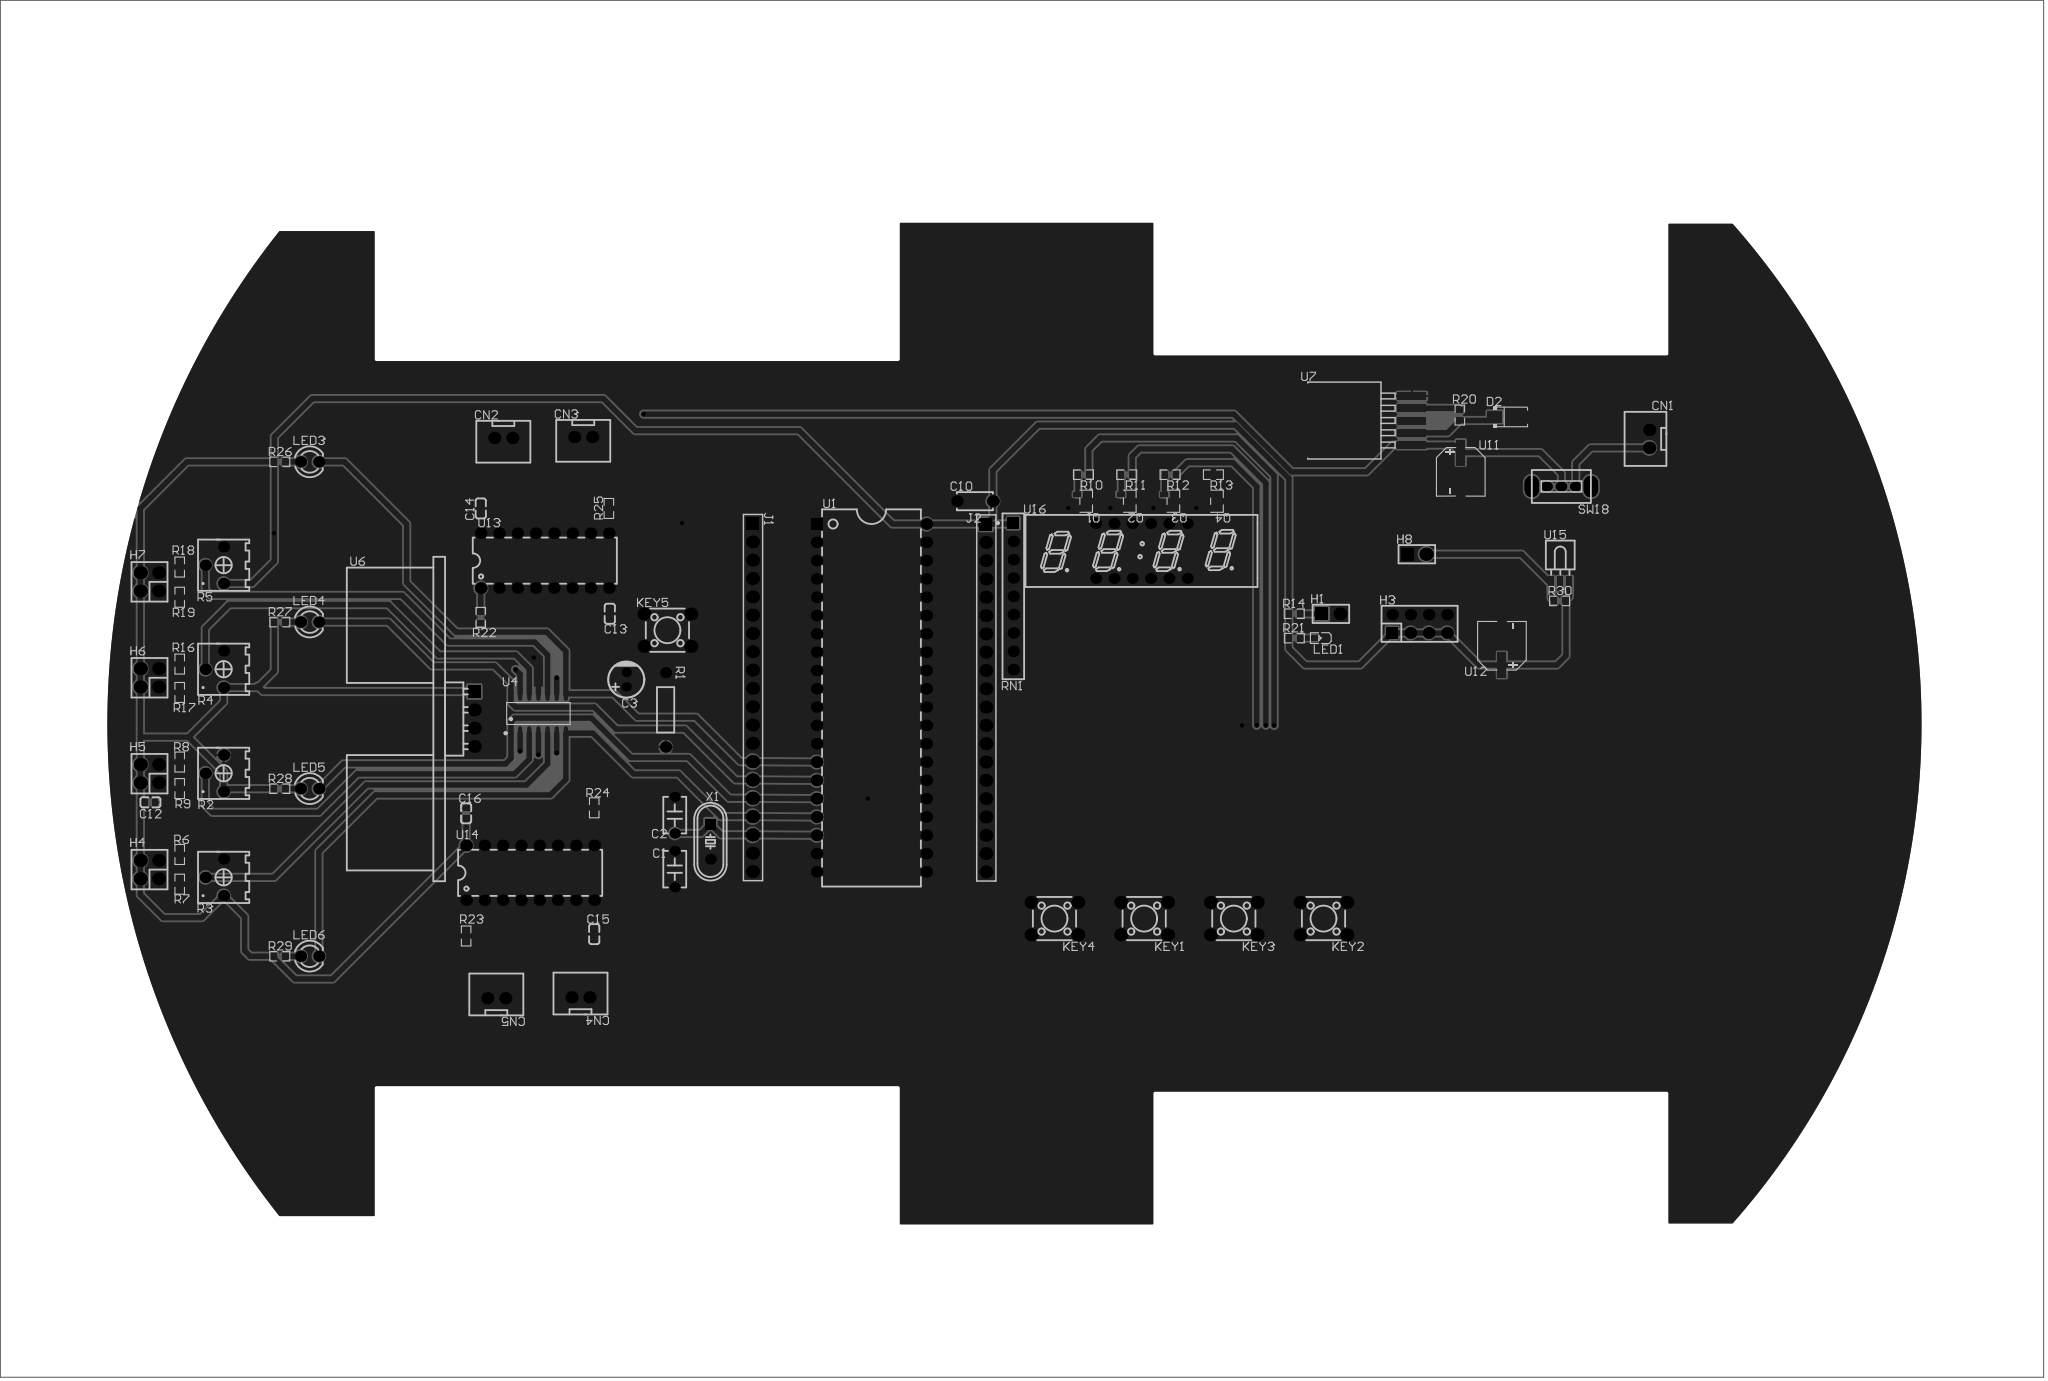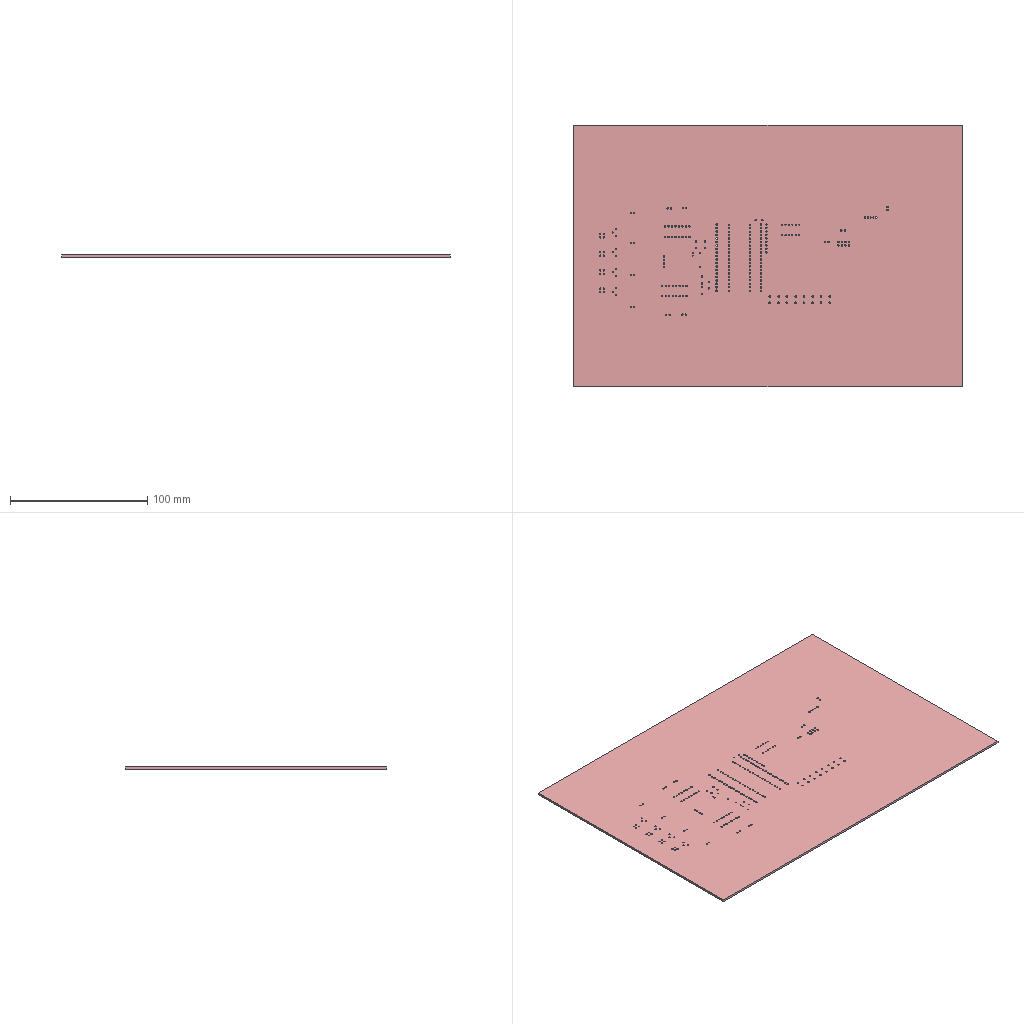Circuit board layout | Altium Designer | box 283.6 x 191 x 1.6 mm
Layer stack:
# Altium Designer layer stack of  (unit mm; dielectric type: 0 none, 1 core, 2 prepreg, 3 surface material)
index,name,kind,layer,copper_thickness_mm,dielectric_type,dielectric_thickness_mm,dielectric_material,dielectric_constant
0,Top Paste Mask Layer,other,,,,,,
1,Top Silkscreen Layer,other,,,,,,
2,Top Solder Mask Layer,dielectric,,,3,0.01,,3.3
3,Top Layer,copper,Top Layer,0.035,,,,
4,Dielectric1,dielectric,,,3,1.51,FR4,4.5
5,Bottom Layer,copper,Bottom Layer,0.035,,,,
6,Bottom Solder Mask Layer,dielectric,,,3,0.01,,3.3
7,Bottom Silkscreen Layer,other,,,,,,
8,Bottom Paste Mask Layer,other,,,,,,
# drill layer pairs: low layer,high layer
drill_pair,Top Layer,Bottom Layer
Part placement:
Designator,Comment,Layer,Footprint,Center-X(mm),Center-Y(mm),Rotation
C1,,TopLayer,CAP-TH_L5.0-W2.5-P5.08-D0.7,163.449,140.335,270
C2,,TopLayer,CAP-TH_L5.0-W2.5-P5.08-D0.7,163.449,147.828,90
C3,,TopLayer,CAP-TH_BD5.0-P2.00-D0.8-FD,156.718,166.624,90
C10,,TopLayer,CAP-TH_L5.0-W2.5-P5.00-D1.0,205.105,191.389,0
C12,104,TopLayer,C0603,90.678,149.606,0
C13,100nF,TopLayer,C0603,154.432,175.768,270
C14,100nF,TopLayer,C0603,136.525,190.373,90
C15,100nF,TopLayer,C0603,152.273,131.318,270
C16,100nF,TopLayer,C0603,134.493,148.082,90
CN1,XH2.54*2P_through-hole,TopLayer,CONN-TH_2P-P2.50-XH2.54-2P,298.704,200.025,270
CN2,XH2.54*2P_through-hole,TopLayer,CONN-TH_2P-P2.50-XH2.54-2P,139.658,200.155,0
CN3,XH2.54*2P_through-hole,TopLayer,CONN-TH_2P-P2.50-XH2.54-2P,150.749,200.279,0
CN4,XH2.54*2P_through-hole,TopLayer,CONN-TH_2P-P2.50-XH2.54-2P,150.368,122.555,180
CN5,XH2.54*2P_through-hole,TopLayer,CONN-TH_2P-P2.50-XH2.54-2P,138.684,122.428,180
D2,SS34,TopLayer,SMA_L4.3-W2.6-LS5.0-RD,279.654,203.073,0
H1,,TopLayer,HDR-TH_2P-P2.54-V-M-1,254.519,175.748,0
H3,,TopLayer,HDR-TH_8P-P2.54-V-F-R2-C4-S2.54-1,266.827,174.371,0
H4,,TopLayer,HDR-TH_4P-P2.54-V-F-R2-C2-S2.54,90.548,140.271,90
H5,,TopLayer,HDR-TH_4P-P2.54-V-F-R2-C2-S2.54,90.548,153.577,90
H6,,TopLayer,HDR-TH_4P-P2.54-V-F-R2-C2-S2.54,90.548,166.884,90
H7,,TopLayer,HDR-TH_4P-P2.54-V-F-R2-C2-S2.54,90.548,180.19,90
H8,,TopLayer,HDR-TH_2P-P2.54-V-M-1,266.446,184.023,0
J1,,TopLayer,HDR-TH_20P-P2.54-V-M-1,174.248,164.14,270
J2,,TopLayer,HDR-TH_20P-P2.54-V-M-1,206.629,164.084,270
KEY1,UK-B0202-G5-160,TopLayer,SW-TH_4P-L6.0-W6.0-P4.50-LS6.5,228.6,133.477,180
KEY2,UK-B0202-G5-160,TopLayer,SW-TH_4P-L6.0-W6.0-P4.50-LS6.5,253.492,133.477,180
KEY3,UK-B0202-G5-160,TopLayer,SW-TH_4P-L6.0-W6.0-P4.50-LS6.5,241.046,133.477,180
KEY4,UK-B0202-G5-160,TopLayer,SW-TH_4P-L6.0-W6.0-P4.50-LS6.5,216.154,133.477,180
KEY5,UK-B0202-G5-160,TopLayer,SW-TH_4P-L6.0-W6.0-P4.50-LS6.5,162.433,173.482,0
LED1,,TopLayer,LED_0603,253.066,172.39,180
LED3,,TopLayer,LED-TH_BD3.0-P2.54-FD,112.789,196.835,0
LED4,,TopLayer,LED-TH_BD3.0-P2.54-FD,112.789,174.61,0
LED5,,TopLayer,LED-TH_BD3.0-P2.54-FD,112.789,151.496,0
LED6,,TopLayer,LED-TH_BD3.0-P2.54-FD,112.789,128.255,0
Q1,S8550,TopLayer,SOT-23-3_L2.9-W1.6-P1.90-LS2.8-BR,220.553,191.376,180
Q2,S8550,TopLayer,SOT-23-3_L2.9-W1.6-P1.90-LS2.8-BR,226.604,191.376,180
Q3,S8550,TopLayer,SOT-23-3_L2.9-W1.6-P1.90-LS2.8-BR,232.655,191.376,180
Q4,S8550,TopLayer,SOT-23-3_L2.9-W1.6-P1.90-LS2.8-BR,238.705,191.376,180
R1,,TopLayer,RES-TH_BD2.4-L6.3-P10.30-D0.6,162.179,162.433,270
R2,-,TopLayer,RES-ADJ-TH_3362P,99.568,153.628,90
R3,-,TopLayer,RES-ADJ-TH_3362P,99.568,139.192,90
R4,-,TopLayer,RES-ADJ-TH_3362P,99.568,168.063,90
R5,-,TopLayer,RES-ADJ-TH_3362P,99.568,182.499,90
R6,10K,TopLayer,R0603,94.742,142.367,90
R7,100,TopLayer,R0603,94.742,138.25,270
R8,10K,TopLayer,R0603,94.742,155.194,90
R9,100,TopLayer,R0603,94.742,151.511,270
R10,1K,TopLayer,R0603,220.172,195.059,180
R11,1K,TopLayer,R0603,226.184,195.059,180
R12,1K,TopLayer,R0603,232.196,195.059,180
R13,1K,TopLayer,R0603,238.208,195.059,180
R14,33,TopLayer,R0603,249.428,175.768,0
R16,10K,TopLayer,R0603,94.742,168.783,90
R17,100,TopLayer,R0603,94.742,164.846,270
R18,10K,TopLayer,R0603,94.742,182.245,90
R19,100,TopLayer,R0603,94.742,178.054,270
R20,33U,TopLayer,R0603,272.415,203.327,270
R21,2K,TopLayer,R0603,249.44,172.383,0
R22,1K,TopLayer,R0603,136.525,175.26,90
R23,1K,TopLayer,R0603,134.493,131.064,90
R24,1K,TopLayer,R0603,152.273,148.844,90
R25,1K,TopLayer,R0603,154.305,190.373,90
R26,1K,TopLayer,R0603,108.636,196.835,0
R27,1K,TopLayer,R0603,108.636,174.61,0
R28,1K,TopLayer,R0603,108.636,151.496,0
R29,1K,TopLayer,R0603,108.636,128.255,0
R30,10K,TopLayer,R0603,286.258,177.546,0
RN1,,TopLayer,RES-ARRAY-TH_9P-P2.54-D1.0,210.439,178.181,270
SW18,,TopLayer,拨动开关,286.504,193.421,180
U1,,TopLayer,DIP-40_L52.0-W13.7-P2.54-LS15.2-BL,190.754,164.084,270
U4,LM324NLM324,TopLayer,SOP-14_L8.6-W3.9-P1.27-LS6.0-BL,144.526,161.925,0
U6,HC-SR04,TopLayer,TH_HC-SR04V,135.636,161.163,270
U7,LM2596SX-5.0/NOPB-YJLTY,TopLayer,TO-263-5_L10.0-W8.4-P1.70-LS15.3-BR,260.223,202.565,0
U11,220uF,TopLayer,CAP-SMD_BD6.3-L6.6-W6.6-LS7.2-FD,272.542,195.453,270
U12,220uF,TopLayer,CAP-SMD_BD6.3-L6.6-W6.6-LS7.2-FD,278.258,171.323,90
U13,L293D,TopLayer,DIP-16_L20.0-W6.4-P2.54-LS7.6-BL,145.415,183.134,0
U14,L293D,TopLayer,DIP-16_L20.0-W6.4-P2.54-LS7.6-BL,143.383,139.827,0
U15,CH0038A_38B/5*5mm/infrared receiver,TopLayer,OPTO-SMD_CH0038A_38B,286.35,179.917,0
U16,0.28 4-digit display,TopLayer,LED-SEG-TH_12P-L32.1-W10.0-P12.7-S7.62-BL,228.23,184.478,0
X1,,TopLayer,HC-49US_L11.5-W4.5-P4.88,168.402,144.145,270
Pad and via stacks:
# Altium Designer via and pad stacks of  (unit mm). Each distinct definition once, with the count of objects using it.
# via: kind,start_layer,end_layer,hole_mm,diameter_mm,mode(0 simple;1 top-mid-bottom;2 full stack),diameter_per_layer,count,example_net
# pad: kind,layer,hole_mm,hole_type(0 round;1 square;2 slot),plating,top_size,top_shape(1 round;2 rect;3 octagon;9 rounded rect),mid_size,bottom_size,mode,footprint,size_per_layer,count,example
pad,Multi-Layer,0.8,0,plated,1.4x1.4,1,1.4x1.4,1.4x1.4,0,CAP-TH_L5.0-W2.5-P5.08-D0.7,,4,C1.1
pad,Multi-Layer,0.8001,0,plated,1.3x1.3,1,1.3x1.3,1.3x1.3,0,CAP-TH_BD5.0-P2.00-D0.8-FD,,2,C3.1
pad,Multi-Layer,1.001,0,plated,1.6x1.6,1,1.6x1.6,1.6x1.6,0,CAP-TH_L5.0-W2.5-P5.00-D1.0,,2,C10.1
pad,Multi-Layer,1.05,0,plated,1.7x1.7,1,1.7x1.7,1.7x1.7,0,CONN-TH_2P-P2.50-XH2.54-2P,,10,CN1.2
pad,Multi-Layer,1.1,0,plated,1.8x1.8,1,1.8x1.8,1.8x1.8,0,HDR-TH_2P-P2.54-V-M-1,,2,H1.2
pad,Multi-Layer,1.1,0,plated,1.8x1.8,2,1.8x1.8,1.8x1.8,0,HDR-TH_2P-P2.54-V-M-1,,2,H1.1
pad,Multi-Layer,1.1,0,plated,1.6x1.6,2,1.6x1.6,1.6x1.6,0,HDR-TH_8P-P2.54-V-F-R2-C4-S2.54-1,,1,H3.1
pad,Multi-Layer,1.1,0,plated,1.6x1.6,1,1.6x1.6,1.6x1.6,0,HDR-TH_8P-P2.54-V-F-R2-C4-S2.54-1,,7,H3.2
pad,Multi-Layer,1,0,plated,1.8x1.8,1,1.8x1.8,1.8x1.8,0,HDR-TH_4P-P2.54-V-F-R2-C2-S2.54,,16,H4.4
pad,Multi-Layer,1.199,0,plated,1.801x1.801,1,1.801x1.801,1.801x1.801,0,HDR-TH_20P-P2.54-V-M-1,,38,J1.20
pad,Multi-Layer,1.199,0,plated,1.801x1.801,2,1.801x1.801,1.801x1.801,0,HDR-TH_20P-P2.54-V-M-1,,2,J1.1
pad,Multi-Layer,1.2,0,plated,1.8x1.8,1,1.8x1.8,1.8x1.8,0,SW-TH_4P-L6.0-W6.0-P4.50-LS6.5,,20,KEY1.1
pad,Multi-Layer,0.9144,0,plated,1.524x1.524,1,1.524x1.524,1.524x1.524,0,LED-TH_BD3.0-P2.54-FD,,8,LED3.1
pad,Multi-Layer,1,0,plated,1.524x1.524,1,1.524x1.524,1.524x1.524,0,RES-TH_BD2.4-L6.3-P10.30-D0.6,,2,R1.1
pad,Multi-Layer,0.762,0,plated,1.524x1.524,1,1.524x1.524,1.524x1.524,0,RES-ADJ-TH_3362P,,12,R2.3
pad,Multi-Layer,1,0,plated,1.6x1.6,2,1.6x1.6,1.6x1.6,0,RES-ARRAY-TH_9P-P2.54-D1.0,,1,RN1.1
pad,Multi-Layer,1,0,plated,1.6x1.6,1,1.6x1.6,1.6x1.6,0,RES-ARRAY-TH_9P-P2.54-D1.0,,8,RN1.2
pad,Multi-Layer,0.8992,0,plated,1.6x1.3,1,1.6x1.3,1.6x1.3,0,\u00B2\u00A6\u00B6\u00AF\u00BF\u00AA\u00B9\u00D8,,3,SW18.1
pad,Multi-Layer,1.3,0,plated,3x1.999,1,3x1.999,3x1.999,0,\u00B2\u00A6\u00B6\u00AF\u00BF\u00AA\u00B9\u00D8,,2,SW18.4
pad,Multi-Layer,0.889,0,plated,1.6x1.6,1,1.6x1.6,1.6x1.6,0,DIP-40_L52.0-W13.7-P2.54-LS15.2-BL,,39,U1.31
pad,Multi-Layer,0.889,0,plated,1.6x1.6,2,1.6x1.6,1.6x1.6,0,DIP-40_L52.0-W13.7-P2.54-LS15.2-BL,,1,U1.1
pad,Multi-Layer,1.001,0,plated,1.8x1.8,1,1.8x1.8,1.8x1.8,0,TH_HC-SR04V,,3,U6.4
pad,Multi-Layer,1.001,0,plated,1.8x1.8,2,1.8x1.8,1.8x1.8,0,TH_HC-SR04V,,1,U6.1
pad,Multi-Layer,1,0,plated,1.6x1.6,1,1.6x1.6,1.6x1.6,0,DIP-16_L20.0-W6.4-P2.54-LS7.6-BL,,32,U13.1
pad,Multi-Layer,0.762,0,plated,1.524x1.524,1,1.524x1.524,1.524x1.524,0,LED-SEG-TH_12P-L32.1-W10.0-P12.7-S7.62-BL,,12,U16.1
pad,Multi-Layer,0.8992,0,plated,1.501x1.501,2,1.501x1.501,1.501x1.501,0,HC-49US_L11.5-W4.5-P4.88,,1,X1.1
pad,Multi-Layer,0.8992,0,plated,1.501x1.501,1,1.501x1.501,1.501x1.501,0,HC-49US_L11.5-W4.5-P4.88,,1,X1.2
pad,Top Layer,0,0,plated,0.8x0.9,2,0.8x0.9,0.8x0.9,0,C0603,,10,C12.2
pad,Top Layer,0,0,plated,2.046x1.62,2,2.046x1.62,2.046x1.62,0,SMA_L4.3-W2.6-LS5.0-RD,,2,D2.2
pad,Top Layer,0,0,plated,0.8001x0.8001,2,0.8001x0.8001,0.8001x0.8001,0,LED_0603,,2,LED1.1
pad,Top Layer,0,0,plated,1.07x0.6,2,1.07x0.6,1.07x0.6,0,SOT-23-3_L2.9-W1.6-P1.90-LS2.8-BR,,12,Q1.1
pad,Top Layer,0,0,plated,0.8065x0.864,2,0.8065x0.864,0.8065x0.864,0,R0603,,48,R6.2
pad,Top Layer,0,0,plated,0.595x1.968,1,0.595x1.968,0.595x1.968,0,SOP-14_L8.6-W3.9-P1.27-LS6.0-BL,,14,U4.1
pad,Top Layer,0,0,plated,4x1.02,2,4x1.02,4x1.02,0,TO-263-5_L10.0-W8.4-P1.70-LS15.3-BR,,5,U7.1
pad,Top Layer,0,0,plated,8.4x10,2,8.4x10,8.4x10,0,TO-263-5_L10.0-W8.4-P1.70-LS15.3-BR,,1,U7.6
pad,Top Layer,0,0,plated,3.5x1.2,2,3.5x1.2,3.5x1.2,0,CAP-SMD_BD6.3-L6.6-W6.6-LS7.2-FD,,4,U11.2
pad,Top Layer,0,0,plated,0.8x2,2,0.8x2,0.8x2,0,OPTO-SMD_CH0038A_38B,,3,U15.3
via,Top Layer,Bottom Layer,0.3048,0.61,0,,18,$1N342
Copper pours:
name,layer,net,type(0 solid;1 hatched;2 none)
Top Layer-GND,Top Layer,GND,0
Bottom Layer-GND,Bottom Layer,GND,0